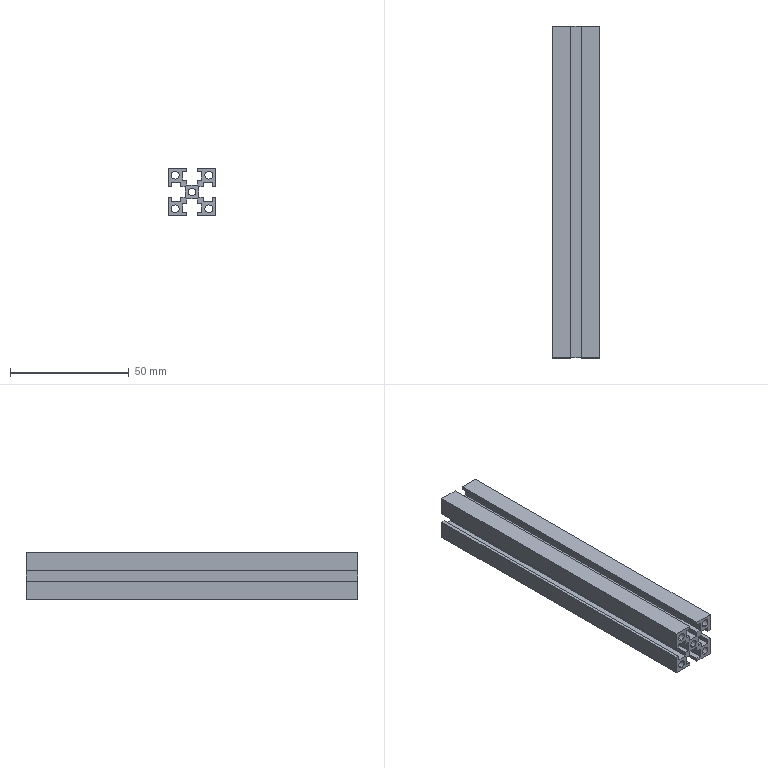Part | STEP file | 20 aluminium profile vertical 1 | 1 solid | 64 faces | box 20 x 140 x 20 mm | volume 24889 mm3 | plane 54 | cylinder 10 | commonest cylinder face diameters 3.3 x10